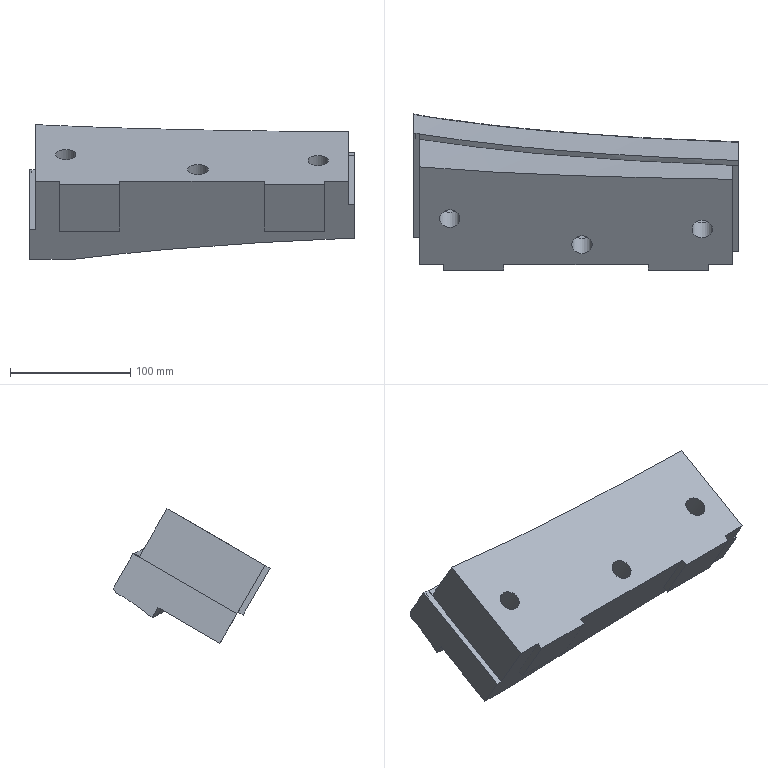Part | NX | features solid 2 | 1 solid | 38 faces | box 270 x 129.945 x 111.971 mm | volume 1492578 mm3 | plane 20 | spline 12 | cylinder 6 | commonest cylinder face diameters 17 x3 25 x3